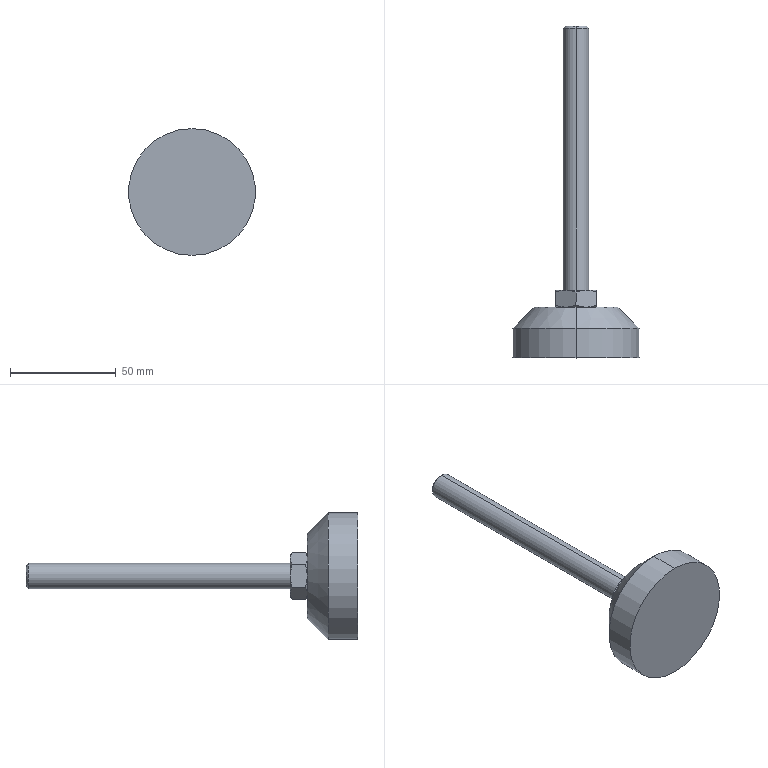Part | STEP file | _GFEEA-D60-M12-L125-1 | 1 solid | 30 faces | box 60 x 157 x 60 mm | volume 76084 mm3 | cone 16 | plane 10 | cylinder 4 | commonest cylinder face diameters 12 x2 60 x2